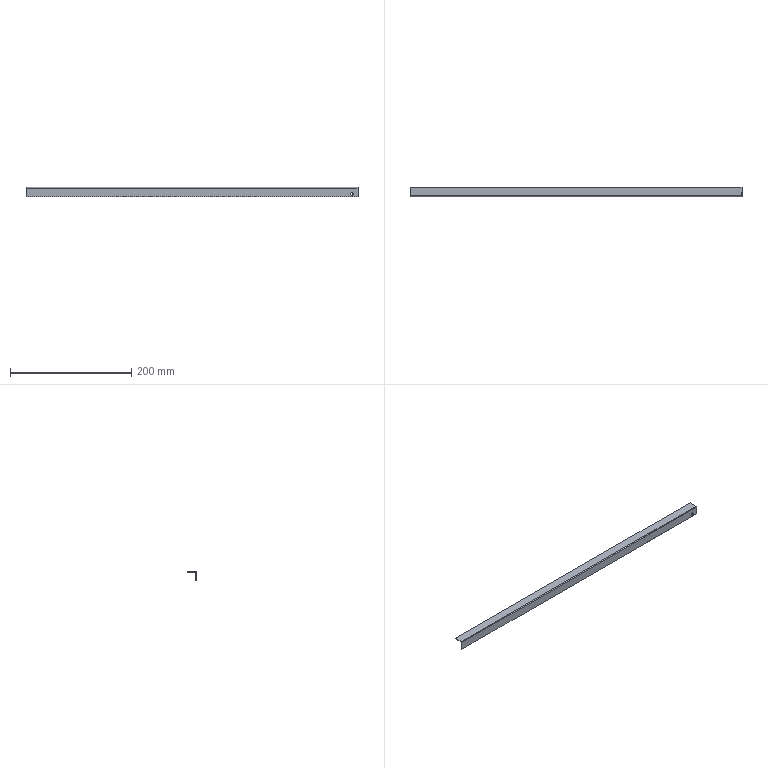Part | SolidWorks | features SplitBody 1 | 1 solid | 16 faces | box 547.1 x 15 x 15 mm | volume 15709 mm3 | plane 12 | cylinder 4 | commonest cylinder face diameters 4.5 x2 0.2 x1 2.2 x1
STEP:
#1=CARTESIAN_POINT('',(-13.95,1437.5,288.));
#2=VERTEX_POINT('',#1);
#3=CARTESIAN_POINT('',(-9.45,1437.5,288.));
#4=VERTEX_POINT('',#3);
#5=CARTESIAN_POINT('',(-11.7,1437.5,288.));
#6=DIRECTION('',(0.,-1.,0.));
#7=DIRECTION('',(1.,0.,0.));
#8=AXIS2_PLACEMENT_3D('',#5,#6,#7);
#9=CIRCLE('',#8,2.25);
#10=EDGE_CURVE('',#2,#4,#9,.T.);
#11=ORIENTED_EDGE('',*,*,#10,.T.);
#12=CARTESIAN_POINT('',(-9.45,1438.5,288.));
#13=VERTEX_POINT('',#12);
#14=CARTESIAN_POINT('',(-9.45,1433.5,288.));
#15=DIRECTION('',(0.,1.,0.));
#16=VECTOR('',#15,1000.);
#17=LINE('',#14,#16);
#18=EDGE_CURVE('',#4,#13,#17,.T.);
#19=ORIENTED_EDGE('',*,*,#18,.T.);
#20=CARTESIAN_POINT('',(-13.95,1438.5,288.));
#21=VERTEX_POINT('',#20);
#22=CARTESIAN_POINT('',(-11.7,1438.5,288.));
#23=DIRECTION('',(0.,1.,0.));
#24=DIRECTION('',(-1.,0.,0.));
#25=AXIS2_PLACEMENT_3D('',#22,#23,#24);
#26=CIRCLE('',#25,2.25);
#27=EDGE_CURVE('',#13,#21,#26,.T.);
#28=ORIENTED_EDGE('',*,*,#27,.T.);
#29=CARTESIAN_POINT('',(-13.95,1433.5,288.));
#30=DIRECTION('',(0.,1.,0.));
#31=VECTOR('',#30,1000.);
#32=LINE('',#29,#31);
#33=EDGE_CURVE('',#2,#21,#32,.T.);
#34=ORIENTED_EDGE('',*,*,#33,.F.);
#35=EDGE_LOOP('',(#11,#19,#28,#34));
#36=FACE_OUTER_BOUND('',#35,.T.);
#37=CARTESIAN_POINT('',(-11.7,1433.5,288.));
#38=DIRECTION('',(0.,1.,0.));
#39=DIRECTION('',(-1.,0.,0.));
#40=AXIS2_PLACEMENT_3D('',#37,#38,#39);
#41=CYLINDRICAL_SURFACE('',#40,2.25);
#42=ADVANCED_FACE('',(#36),#41,.F.);
#43=CARTESIAN_POINT('',(-548.8,1437.5,297.7));
#44=VERTEX_POINT('',#43);
#45=CARTESIAN_POINT('',(-548.8,1438.5,297.7));
#46=VERTEX_POINT('',#45);
#47=CARTESIAN_POINT('',(-548.8,1437.5,297.7));
#48=DIRECTION('',(0.,1.,0.));
#49=VECTOR('',#48,1000.);
#50=LINE('',#47,#49);
#51=EDGE_CURVE('',#44,#46,#50,.T.);
#52=ORIENTED_EDGE('',*,*,#51,.F.);
#53=CARTESIAN_POINT('',(-548.8,1438.6,298.8));
#54=VERTEX_POINT('',#53);
#55=CARTESIAN_POINT('',(-548.8,1438.6,297.7));
#56=DIRECTION('',(-1.,0.,0.));
#57=DIRECTION('',(0.,0.,-1.));
#58=AXIS2_PLACEMENT_3D('',#55,#56,#57);
#59=CIRCLE('',#58,1.1);
#60=EDGE_CURVE('',#44,#54,#59,.T.);
#61=ORIENTED_EDGE('',*,*,#60,.T.);
#62=CARTESIAN_POINT('',(-548.8,1438.6,297.8));
#63=VERTEX_POINT('',#62);
#64=CARTESIAN_POINT('',(-548.8,1438.6,297.8));
#65=DIRECTION('',(0.,0.,1.));
#66=VECTOR('',#65,1000.);
#67=LINE('',#64,#66);
#68=EDGE_CURVE('',#63,#54,#67,.T.);
#69=ORIENTED_EDGE('',*,*,#68,.F.);
#70=CARTESIAN_POINT('',(-548.8,1438.6,297.7));
#71=DIRECTION('',(-1.,0.,0.));
#72=DIRECTION('',(0.,0.,-1.));
#73=AXIS2_PLACEMENT_3D('',#70,#71,#72);
#74=CIRCLE('',#73,0.1);
#75=EDGE_CURVE('',#46,#63,#74,.T.);
#76=ORIENTED_EDGE('',*,*,#75,.F.);
#77=EDGE_LOOP('',(#52,#61,#69,#76));
#78=FACE_OUTER_BOUND('',#77,.T.);
#79=CARTESIAN_POINT('',(-548.8,1437.5,297.7));
#80=DIRECTION('',(-1.,0.,0.));
#81=DIRECTION('',(0.,0.,1.));
#82=AXIS2_PLACEMENT_3D('',#79,#80,#81);
#83=PLANE('',#82);
#84=ADVANCED_FACE('',(#78),#83,.T.);
#85=CARTESIAN_POINT('',(-548.8,1437.5,283.8));
#86=VERTEX_POINT('',#85);
#87=CARTESIAN_POINT('',(-548.8,1437.5,283.8));
#88=DIRECTION('',(0.,0.,1.));
#89=VECTOR('',#88,1000.);
#90=LINE('',#87,#89);
#91=EDGE_CURVE('',#86,#44,#90,.T.);
#92=ORIENTED_EDGE('',*,*,#91,.T.);
#93=ORIENTED_EDGE('',*,*,#51,.T.);
#94=CARTESIAN_POINT('',(-548.8,1438.5,283.8));
#95=VERTEX_POINT('',#94);
#96=CARTESIAN_POINT('',(-548.8,1438.5,283.8));
#97=DIRECTION('',(0.,0.,1.));
#98=VECTOR('',#97,1000.);
#99=LINE('',#96,#98);
#100=EDGE_CURVE('',#95,#46,#99,.T.);
#101=ORIENTED_EDGE('',*,*,#100,.F.);
#102=CARTESIAN_POINT('',(-548.8,1438.5,283.8));
#103=DIRECTION('',(0.,-1.,0.));
#104=VECTOR('',#103,1000.);
#105=LINE('',#102,#104);
#106=EDGE_CURVE('',#95,#86,#105,.T.);
#107=ORIENTED_EDGE('',*,*,#106,.T.);
#108=EDGE_LOOP('',(#92,#93,#101,#107));
#109=FACE_OUTER_BOUND('',#108,.T.);
#110=CARTESIAN_POINT('',(-548.8,1438.6,297.8));
#111=DIRECTION('',(-1.,0.,0.));
#112=DIRECTION('',(0.,0.,1.));
#113=AXIS2_PLACEMENT_3D('',#110,#111,#112);
#114=PLANE('',#113);
#115=ADVANCED_FACE('',(#109),#114,.T.);
#116=CARTESIAN_POINT('',(-1.7,1452.5,297.8));
#117=VERTEX_POINT('',#116);
#118=CARTESIAN_POINT('',(-1.7,1438.6,297.8));
#119=VERTEX_POINT('',#118);
#120=CARTESIAN_POINT('',(-1.7,1437.5,297.8));
#121=DIRECTION('',(0.,-1.,0.));
#122=VECTOR('',#121,1000.);
#123=LINE('',#120,#122);
#124=EDGE_CURVE('',#117,#119,#123,.T.);
#125=ORIENTED_EDGE('',*,*,#124,.T.);
#126=CARTESIAN_POINT('',(19.513,1438.6,297.8));
#127=DIRECTION('',(-1.,0.,0.));
#128=VECTOR('',#127,1000.);
#129=LINE('',#126,#128);
#130=EDGE_CURVE('',#119,#63,#129,.T.);
#131=ORIENTED_EDGE('',*,*,#130,.T.);
#132=CARTESIAN_POINT('',(-548.8,1452.5,297.8));
#133=VERTEX_POINT('',#132);
#134=CARTESIAN_POINT('',(-548.8,1437.5,297.8));
#135=DIRECTION('',(0.,1.,0.));
#136=VECTOR('',#135,1000.);
#137=LINE('',#134,#136);
#138=EDGE_CURVE('',#63,#133,#137,.T.);
#139=ORIENTED_EDGE('',*,*,#138,.T.);
#140=CARTESIAN_POINT('',(19.513,1452.5,297.8));
#141=DIRECTION('',(-1.,0.,0.));
#142=VECTOR('',#141,1000.);
#143=LINE('',#140,#142);
#144=EDGE_CURVE('',#117,#133,#143,.T.);
#145=ORIENTED_EDGE('',*,*,#144,.F.);
#146=EDGE_LOOP('',(#125,#131,#139,#145));
#147=FACE_OUTER_BOUND('',#146,.T.);
#148=CARTESIAN_POINT('',(19.513,1437.5,297.8));
#149=DIRECTION('',(0.,0.,1.));
#150=DIRECTION('',(1.,0.,0.));
#151=AXIS2_PLACEMENT_3D('',#148,#149,#150);
#152=PLANE('',#151);
#153=ADVANCED_FACE('',(#147),#152,.F.);
#154=CARTESIAN_POINT('',(-1.7,1452.5,298.8));
#155=VERTEX_POINT('',#154);
#156=CARTESIAN_POINT('',(-548.8,1452.5,298.8));
#157=VERTEX_POINT('',#156);
#158=CARTESIAN_POINT('',(19.513,1452.5,298.8));
#159=DIRECTION('',(-1.,0.,0.));
#160=VECTOR('',#159,1000.);
#161=LINE('',#158,#160);
#162=EDGE_CURVE('',#155,#157,#161,.T.);
#163=ORIENTED_EDGE('',*,*,#162,.F.);
#164=CARTESIAN_POINT('',(-1.7,1452.5,297.8));
#165=DIRECTION('',(0.,0.,1.));
#166=VECTOR('',#165,1000.);
#167=LINE('',#164,#166);
#168=EDGE_CURVE('',#117,#155,#167,.T.);
#169=ORIENTED_EDGE('',*,*,#168,.F.);
#170=ORIENTED_EDGE('',*,*,#144,.T.);
#171=CARTESIAN_POINT('',(-548.8,1452.5,298.8));
#172=DIRECTION('',(0.,0.,-1.));
#173=VECTOR('',#172,1000.);
#174=LINE('',#171,#173);
#175=EDGE_CURVE('',#157,#133,#174,.T.);
#176=ORIENTED_EDGE('',*,*,#175,.F.);
#177=EDGE_LOOP('',(#163,#169,#170,#176));
#178=FACE_OUTER_BOUND('',#177,.T.);
#179=CARTESIAN_POINT('',(19.513,1452.5,298.8));
#180=DIRECTION('',(0.,1.,0.));
#181=DIRECTION('',(-1.,0.,0.));
#182=AXIS2_PLACEMENT_3D('',#179,#180,#181);
#183=PLANE('',#182);
#184=ADVANCED_FACE('',(#178),#183,.T.);
#185=CARTESIAN_POINT('',(-1.7,1438.6,298.8));
#186=VERTEX_POINT('',#185);
#187=CARTESIAN_POINT('',(19.513,1438.6,298.8));
#188=DIRECTION('',(-1.,0.,0.));
#189=VECTOR('',#188,1000.);
#190=LINE('',#187,#189);
#191=EDGE_CURVE('',#186,#54,#190,.T.);
#192=ORIENTED_EDGE('',*,*,#191,.F.);
#193=CARTESIAN_POINT('',(-1.7,1437.5,298.8));
#194=DIRECTION('',(0.,-1.,0.));
#195=VECTOR('',#194,1000.);
#196=LINE('',#193,#195);
#197=EDGE_CURVE('',#155,#186,#196,.T.);
#198=ORIENTED_EDGE('',*,*,#197,.F.);
#199=ORIENTED_EDGE('',*,*,#162,.T.);
#200=CARTESIAN_POINT('',(-548.8,1437.5,298.8));
#201=DIRECTION('',(0.,1.,0.));
#202=VECTOR('',#201,1000.);
#203=LINE('',#200,#202);
#204=EDGE_CURVE('',#54,#157,#203,.T.);
#205=ORIENTED_EDGE('',*,*,#204,.F.);
#206=EDGE_LOOP('',(#192,#198,#199,#205));
#207=FACE_OUTER_BOUND('',#206,.T.);
#208=CARTESIAN_POINT('',(19.513,1437.5,298.8));
#209=DIRECTION('',(0.,0.,1.));
#210=DIRECTION('',(1.,0.,0.));
#211=AXIS2_PLACEMENT_3D('',#208,#209,#210);
#212=PLANE('',#211);
#213=ADVANCED_FACE('',(#207),#212,.T.);
#214=CARTESIAN_POINT('',(-1.7,1437.5,297.7));
#215=VERTEX_POINT('',#214);
#216=CARTESIAN_POINT('',(19.513,1437.5,297.7));
#217=DIRECTION('',(-1.,0.,0.));
#218=VECTOR('',#217,1000.);
#219=LINE('',#216,#218);
#220=EDGE_CURVE('',#215,#44,#219,.T.);
#221=ORIENTED_EDGE('',*,*,#220,.F.);
#222=CARTESIAN_POINT('',(-1.7,1438.6,297.7));
#223=DIRECTION('',(1.,0.,0.));
#224=DIRECTION('',(0.,0.,-1.));
#225=AXIS2_PLACEMENT_3D('',#222,#223,#224);
#226=CIRCLE('',#225,1.1);
#227=EDGE_CURVE('',#186,#215,#226,.T.);
#228=ORIENTED_EDGE('',*,*,#227,.F.);
#229=ORIENTED_EDGE('',*,*,#191,.T.);
#230=ORIENTED_EDGE('',*,*,#60,.F.);
#231=EDGE_LOOP('',(#221,#228,#229,#230));
#232=FACE_OUTER_BOUND('',#231,.T.);
#233=CARTESIAN_POINT('',(19.513,1438.6,297.7));
#234=DIRECTION('',(-1.,0.,0.));
#235=DIRECTION('',(0.,0.,1.));
#236=AXIS2_PLACEMENT_3D('',#233,#234,#235);
#237=CYLINDRICAL_SURFACE('',#236,1.1);
#238=ADVANCED_FACE('',(#232),#237,.T.);
#239=ORIENTED_EDGE('',*,*,#10,.F.);
#240=CARTESIAN_POINT('',(-11.7,1437.5,288.));
#241=DIRECTION('',(0.,-1.,0.));
#242=DIRECTION('',(1.,0.,0.));
#243=AXIS2_PLACEMENT_3D('',#240,#241,#242);
#244=CIRCLE('',#243,2.25);
#245=EDGE_CURVE('',#4,#2,#244,.T.);
#246=ORIENTED_EDGE('',*,*,#245,.F.);
#247=EDGE_LOOP('',(#239,#246));
#248=FACE_BOUND('',#247,.T.);
#249=CARTESIAN_POINT('',(-1.7,1437.5,283.8));
#250=VERTEX_POINT('',#249);
#251=CARTESIAN_POINT('',(19.513,1437.5,283.8));
#252=DIRECTION('',(-1.,0.,0.));
#253=VECTOR('',#252,1000.);
#254=LINE('',#251,#253);
#255=EDGE_CURVE('',#250,#86,#254,.T.);
#256=ORIENTED_EDGE('',*,*,#255,.F.);
#257=CARTESIAN_POINT('',(-1.7,1437.5,283.8));
#258=DIRECTION('',(0.,0.,-1.));
#259=VECTOR('',#258,1000.);
#260=LINE('',#257,#259);
#261=EDGE_CURVE('',#215,#250,#260,.T.);
#262=ORIENTED_EDGE('',*,*,#261,.F.);
#263=ORIENTED_EDGE('',*,*,#220,.T.);
#264=ORIENTED_EDGE('',*,*,#91,.F.);
#265=EDGE_LOOP('',(#256,#262,#263,#264));
#266=FACE_OUTER_BOUND('',#265,.T.);
#267=CARTESIAN_POINT('',(19.513,1437.5,283.8));
#268=DIRECTION('',(0.,-1.,0.));
#269=DIRECTION('',(1.,0.,0.));
#270=AXIS2_PLACEMENT_3D('',#267,#268,#269);
#271=PLANE('',#270);
#272=ADVANCED_FACE('',(#248,#266),#271,.T.);
#273=CARTESIAN_POINT('',(-1.7,1438.5,283.8));
#274=VERTEX_POINT('',#273);
#275=CARTESIAN_POINT('',(19.513,1438.5,283.8));
#276=DIRECTION('',(-1.,0.,0.));
#277=VECTOR('',#276,1000.);
#278=LINE('',#275,#277);
#279=EDGE_CURVE('',#274,#95,#278,.T.);
#280=ORIENTED_EDGE('',*,*,#279,.F.);
#281=CARTESIAN_POINT('',(-1.7,1438.5,283.8));
#282=DIRECTION('',(0.,-1.,0.));
#283=VECTOR('',#282,1000.);
#284=LINE('',#281,#283);
#285=EDGE_CURVE('',#274,#250,#284,.T.);
#286=ORIENTED_EDGE('',*,*,#285,.T.);
#287=ORIENTED_EDGE('',*,*,#255,.T.);
#288=ORIENTED_EDGE('',*,*,#106,.F.);
#289=EDGE_LOOP('',(#280,#286,#287,#288));
#290=FACE_OUTER_BOUND('',#289,.T.);
#291=CARTESIAN_POINT('',(19.513,1438.5,283.8));
#292=DIRECTION('',(0.,0.,-1.));
#293=DIRECTION('',(-1.,0.,0.));
#294=AXIS2_PLACEMENT_3D('',#291,#292,#293);
#295=PLANE('',#294);
#296=ADVANCED_FACE('',(#290),#295,.T.);
#297=CARTESIAN_POINT('',(-11.7,1438.5,288.));
#298=DIRECTION('',(0.,1.,0.));
#299=DIRECTION('',(-1.,0.,0.));
#300=AXIS2_PLACEMENT_3D('',#297,#298,#299);
#301=CIRCLE('',#300,2.25);
#302=EDGE_CURVE('',#21,#13,#301,.T.);
#303=ORIENTED_EDGE('',*,*,#302,.F.);
#304=ORIENTED_EDGE('',*,*,#27,.F.);
#305=EDGE_LOOP('',(#303,#304));
#306=FACE_BOUND('',#305,.T.);
#307=CARTESIAN_POINT('',(-1.7,1438.5,297.7));
#308=VERTEX_POINT('',#307);
#309=CARTESIAN_POINT('',(-1.7,1438.5,283.8));
#310=DIRECTION('',(0.,0.,-1.));
#311=VECTOR('',#310,1000.);
#312=LINE('',#309,#311);
#313=EDGE_CURVE('',#308,#274,#312,.T.);
#314=ORIENTED_EDGE('',*,*,#313,.T.);
#315=ORIENTED_EDGE('',*,*,#279,.T.);
#316=ORIENTED_EDGE('',*,*,#100,.T.);
#317=CARTESIAN_POINT('',(19.513,1438.5,297.7));
#318=DIRECTION('',(-1.,0.,0.));
#319=VECTOR('',#318,1000.);
#320=LINE('',#317,#319);
#321=EDGE_CURVE('',#308,#46,#320,.T.);
#322=ORIENTED_EDGE('',*,*,#321,.F.);
#323=EDGE_LOOP('',(#314,#315,#316,#322));
#324=FACE_OUTER_BOUND('',#323,.T.);
#325=CARTESIAN_POINT('',(19.513,1438.5,283.8));
#326=DIRECTION('',(0.,-1.,0.));
#327=DIRECTION('',(1.,0.,0.));
#328=AXIS2_PLACEMENT_3D('',#325,#326,#327);
#329=PLANE('',#328);
#330=ADVANCED_FACE('',(#306,#324),#329,.F.);
#331=CARTESIAN_POINT('',(-1.7,1438.6,297.7));
#332=DIRECTION('',(1.,0.,0.));
#333=DIRECTION('',(0.,0.,1.));
#334=AXIS2_PLACEMENT_3D('',#331,#332,#333);
#335=CIRCLE('',#334,0.1);
#336=EDGE_CURVE('',#119,#308,#335,.T.);
#337=ORIENTED_EDGE('',*,*,#336,.T.);
#338=ORIENTED_EDGE('',*,*,#321,.T.);
#339=ORIENTED_EDGE('',*,*,#75,.T.);
#340=ORIENTED_EDGE('',*,*,#130,.F.);
#341=EDGE_LOOP('',(#337,#338,#339,#340));
#342=FACE_OUTER_BOUND('',#341,.T.);
#343=CARTESIAN_POINT('',(19.513,1438.6,297.7));
#344=DIRECTION('',(-1.,0.,0.));
#345=DIRECTION('',(0.,0.,1.));
#346=AXIS2_PLACEMENT_3D('',#343,#344,#345);
#347=CYLINDRICAL_SURFACE('',#346,0.1);
#348=ADVANCED_FACE('',(#342),#347,.F.);
#349=ORIENTED_EDGE('',*,*,#138,.F.);
#350=ORIENTED_EDGE('',*,*,#68,.T.);
#351=ORIENTED_EDGE('',*,*,#204,.T.);
#352=ORIENTED_EDGE('',*,*,#175,.T.);
#353=EDGE_LOOP('',(#349,#350,#351,#352));
#354=FACE_OUTER_BOUND('',#353,.T.);
#355=CARTESIAN_POINT('',(-548.8,1438.6,297.7));
#356=DIRECTION('',(1.,0.,0.));
#357=DIRECTION('',(0.,0.,-1.));
#358=AXIS2_PLACEMENT_3D('',#355,#356,#357);
#359=PLANE('',#358);
#360=ADVANCED_FACE('',(#354),#359,.F.);
#361=CARTESIAN_POINT('',(-1.7,1438.6,297.8));
#362=DIRECTION('',(0.,0.,1.));
#363=VECTOR('',#362,1000.);
#364=LINE('',#361,#363);
#365=EDGE_CURVE('',#119,#186,#364,.T.);
#366=ORIENTED_EDGE('',*,*,#365,.F.);
#367=ORIENTED_EDGE('',*,*,#124,.F.);
#368=ORIENTED_EDGE('',*,*,#168,.T.);
#369=ORIENTED_EDGE('',*,*,#197,.T.);
#370=EDGE_LOOP('',(#366,#367,#368,#369));
#371=FACE_OUTER_BOUND('',#370,.T.);
#372=CARTESIAN_POINT('',(-1.7,1437.5,297.8));
#373=DIRECTION('',(-1.,0.,0.));
#374=DIRECTION('',(0.,-1.,0.));
#375=AXIS2_PLACEMENT_3D('',#372,#373,#374);
#376=PLANE('',#375);
#377=ADVANCED_FACE('',(#371),#376,.F.);
#378=ORIENTED_EDGE('',*,*,#285,.F.);
#379=ORIENTED_EDGE('',*,*,#313,.F.);
#380=CARTESIAN_POINT('',(-1.7,1438.5,297.7));
#381=DIRECTION('',(0.,-1.,0.));
#382=VECTOR('',#381,1000.);
#383=LINE('',#380,#382);
#384=EDGE_CURVE('',#308,#215,#383,.T.);
#385=ORIENTED_EDGE('',*,*,#384,.T.);
#386=ORIENTED_EDGE('',*,*,#261,.T.);
#387=EDGE_LOOP('',(#378,#379,#385,#386));
#388=FACE_OUTER_BOUND('',#387,.T.);
#389=CARTESIAN_POINT('',(-1.7,1438.5,283.8));
#390=DIRECTION('',(-1.,0.,0.));
#391=DIRECTION('',(0.,0.,-1.));
#392=AXIS2_PLACEMENT_3D('',#389,#390,#391);
#393=PLANE('',#392);
#394=ADVANCED_FACE('',(#388),#393,.F.);
#395=ORIENTED_EDGE('',*,*,#227,.T.);
#396=ORIENTED_EDGE('',*,*,#384,.F.);
#397=ORIENTED_EDGE('',*,*,#336,.F.);
#398=ORIENTED_EDGE('',*,*,#365,.T.);
#399=EDGE_LOOP('',(#395,#396,#397,#398));
#400=FACE_OUTER_BOUND('',#399,.T.);
#401=CARTESIAN_POINT('',(-1.7,1438.6,297.7));
#402=DIRECTION('',(1.,0.,0.));
#403=DIRECTION('',(0.,0.,-1.));
#404=AXIS2_PLACEMENT_3D('',#401,#402,#403);
#405=PLANE('',#404);
#406=ADVANCED_FACE('',(#400),#405,.T.);
#407=ORIENTED_EDGE('',*,*,#18,.F.);
#408=ORIENTED_EDGE('',*,*,#245,.T.);
#409=ORIENTED_EDGE('',*,*,#33,.T.);
#410=ORIENTED_EDGE('',*,*,#302,.T.);
#411=EDGE_LOOP('',(#407,#408,#409,#410));
#412=FACE_OUTER_BOUND('',#411,.T.);
#413=CARTESIAN_POINT('',(-11.7,1433.5,288.));
#414=DIRECTION('',(0.,1.,0.));
#415=DIRECTION('',(-1.,0.,0.));
#416=AXIS2_PLACEMENT_3D('',#413,#414,#415);
#417=CYLINDRICAL_SURFACE('',#416,2.25);
#418=ADVANCED_FACE('',(#412),#417,.F.);
#419=CLOSED_SHELL('',(#42,#84,#115,#153,#184,#213,#238,#272,#296,#330,#348,#360,#377,#394,#406,#418));
#420=MANIFOLD_SOLID_BREP('',#419);
#421=CARTESIAN_POINT('',(0.,0.,0.));
#422=DIRECTION('',(0.,0.,1.));
#423=DIRECTION('',(1.,0.,0.));
#424=AXIS2_PLACEMENT_3D('',#421,#422,#423);
#425=(LENGTH_UNIT()NAMED_UNIT(*)SI_UNIT(.MILLI.,.METRE.));
#426=UNCERTAINTY_MEASURE_WITH_UNIT(LENGTH_MEASURE(0.00001),#425,'','');
#427=(NAMED_UNIT(*)PLANE_ANGLE_UNIT()SI_UNIT($,.RADIAN.));
#428=(NAMED_UNIT(*)SI_UNIT($,.STERADIAN.)SOLID_ANGLE_UNIT());
#429=(GEOMETRIC_REPRESENTATION_CONTEXT(3)GLOBAL_UNCERTAINTY_ASSIGNED_CONTEXT((#426))GLOBAL_UNIT_ASSIGNED_CONTEXT((#425,#427,#428))REPRESENTATION_CONTEXT('',''));
#430=ADVANCED_BREP_SHAPE_REPRESENTATION('',(#420,#424),#429);